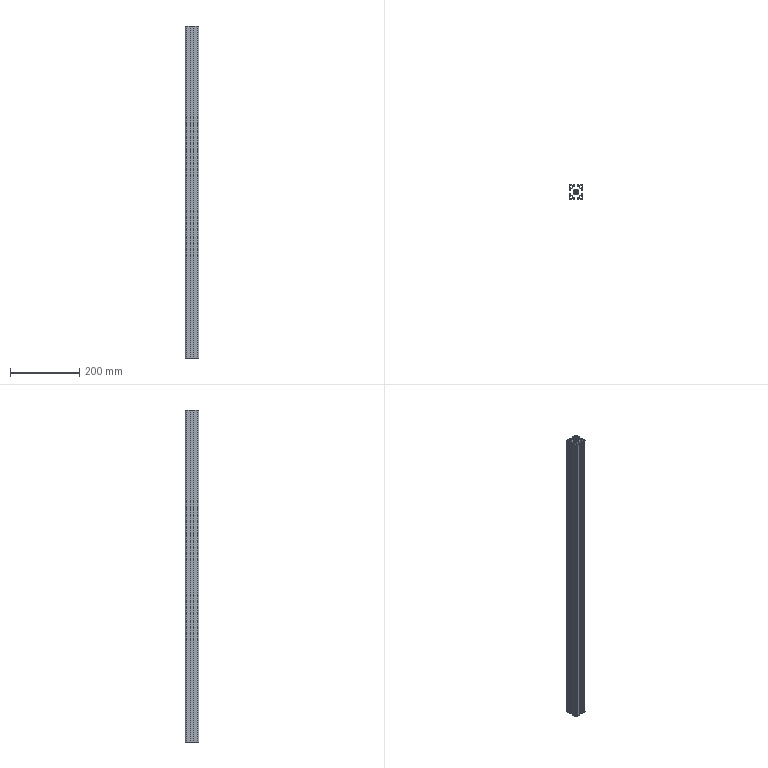Part | SolidWorks | features BaseBody 1, MoveFace 1 | 1 solid | 129 faces | box 40 x 40 x 956 mm | volume 413693 mm3 | plane 102 | cylinder 27 | commonest cylinder face diameters 2 x8 1.5 x6 6.8 x5 6.6 x4 9 x4